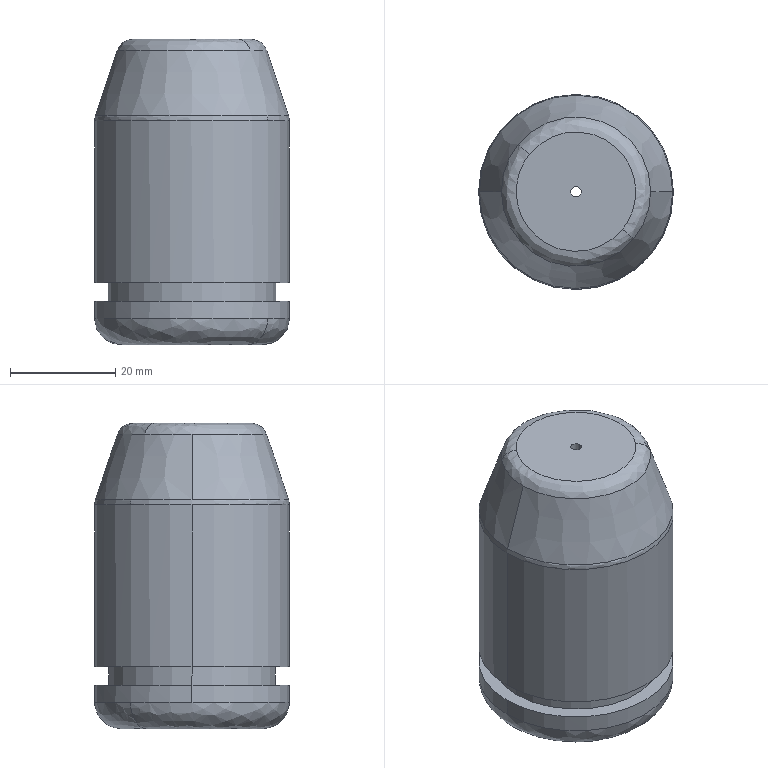Part | SolidWorks | features BaseBody 1 | 1 solid | 23 faces | box 37 x 37 x 58 mm | volume 55664 mm3 | cylinder 10 | spline 6 | plane 5 | cone 2 | commonest cylinder face diameters 37 x4 2 x2 5 x2 31.8 x2
STEP:
#1=CARTESIAN_POINT('',(495.143,-122.508,308.325));
#2=VERTEX_POINT('',#1);
#3=CARTESIAN_POINT('',(527.996,-134.18,308.325));
#4=VERTEX_POINT('',#3);
#5=CARTESIAN_POINT('',(509.496,-134.18,308.325));
#6=DIRECTION('',(-0.000000024,0.000000004,-1.));
#7=DIRECTION('',(-1.,0.,0.000000024));
#8=AXIS2_PLACEMENT_3D('',#5,#6,#7);
#9=CIRCLE('',#8,18.5);
#10=EDGE_CURVE('',#2,#4,#9,.T.);
#11=ORIENTED_EDGE('',*,*,#10,.F.);
#12=CARTESIAN_POINT('',(495.263,-122.605,309.274));
#13=VERTEX_POINT('',#12);
#14=CARTESIAN_POINT('',(497.471,-124.401,308.325));
#15=DIRECTION('',(0.6309,0.7758,-0.000000012));
#16=DIRECTION('',(-0.7758,0.6309,0.000000021));
#17=AXIS2_PLACEMENT_3D('',#14,#15,#16);
#18=CIRCLE('',#17,3.);
#19=EDGE_CURVE('',#2,#13,#18,.T.);
#20=ORIENTED_EDGE('',*,*,#19,.T.);
#21=CARTESIAN_POINT('',(527.842,-134.18,309.274));
#22=VERTEX_POINT('',#21);
#23=CARTESIAN_POINT('',(509.496,-134.18,309.274));
#24=DIRECTION('',(-0.000000024,0.000000004,-1.));
#25=DIRECTION('',(0.7758,-0.6309,-0.000000021));
#26=AXIS2_PLACEMENT_3D('',#23,#24,#25);
#27=CIRCLE('',#26,18.346);
#28=EDGE_CURVE('',#13,#22,#27,.T.);
#29=ORIENTED_EDGE('',*,*,#28,.T.);
#30=CARTESIAN_POINT('',(523.73,-145.756,309.274));
#31=VERTEX_POINT('',#30);
#32=CARTESIAN_POINT('',(509.496,-134.18,309.274));
#33=DIRECTION('',(-0.000000024,0.000000004,-1.));
#34=DIRECTION('',(0.7758,-0.6309,-0.000000021));
#35=AXIS2_PLACEMENT_3D('',#32,#33,#34);
#36=CIRCLE('',#35,18.346);
#37=EDGE_CURVE('',#22,#31,#36,.T.);
#38=ORIENTED_EDGE('',*,*,#37,.T.);
#39=CARTESIAN_POINT('',(523.849,-145.853,308.325));
#40=VERTEX_POINT('',#39);
#41=CARTESIAN_POINT('',(521.522,-143.96,308.325));
#42=DIRECTION('',(-0.6309,-0.7758,0.000000012));
#43=DIRECTION('',(0.7758,-0.6309,-0.000000021));
#44=AXIS2_PLACEMENT_3D('',#41,#42,#43);
#45=CIRCLE('',#44,3.);
#46=EDGE_CURVE('',#40,#31,#45,.T.);
#47=ORIENTED_EDGE('',*,*,#46,.F.);
#48=CARTESIAN_POINT('',(509.496,-134.18,308.325));
#49=DIRECTION('',(-0.000000024,0.000000004,-1.));
#50=DIRECTION('',(-1.,0.,0.000000024));
#51=AXIS2_PLACEMENT_3D('',#48,#49,#50);
#52=CIRCLE('',#51,18.5);
#53=EDGE_CURVE('',#4,#40,#52,.T.);
#54=ORIENTED_EDGE('',*,*,#53,.F.);
#55=EDGE_LOOP('',(#11,#20,#29,#38,#47,#54));
#56=FACE_OUTER_BOUND('',#55,.T.);
#57=CARTESIAN_POINT('',(495.143,-122.508,308.325));
#58=CARTESIAN_POINT('',(518.488,-93.802,308.325));
#59=CARTESIAN_POINT('',(547.194,-117.147,308.325));
#60=CARTESIAN_POINT('',(523.849,-145.853,308.325));
#61=CARTESIAN_POINT('',(495.143,-122.508,308.648));
#62=CARTESIAN_POINT('',(518.488,-93.802,308.648));
#63=CARTESIAN_POINT('',(547.194,-117.147,308.648));
#64=CARTESIAN_POINT('',(523.849,-145.853,308.648));
#65=CARTESIAN_POINT('',(495.183,-122.541,308.967));
#66=CARTESIAN_POINT('',(518.462,-93.915,308.967));
#67=CARTESIAN_POINT('',(547.088,-117.194,308.967));
#68=CARTESIAN_POINT('',(523.809,-145.82,308.967));
#69=CARTESIAN_POINT('',(495.263,-122.605,309.274));
#70=CARTESIAN_POINT('',(518.413,-94.138,309.274));
#71=CARTESIAN_POINT('',(546.88,-117.288,309.274));
#72=CARTESIAN_POINT('',(523.73,-145.756,309.274));
#73=(BOUNDED_SURFACE()B_SPLINE_SURFACE(3,3,((#57,#58,#59,#60),(#61,#62,#63,#64),(#65,#66,#67,#68),(#69,#70,#71,#72)),.UNSPECIFIED.,.F.,.F.,.T.)B_SPLINE_SURFACE_WITH_KNOTS((4,4),(4,4),(0.,1.),(0.,1.),.UNSPECIFIED.)GEOMETRIC_REPRESENTATION_ITEM()RATIONAL_B_SPLINE_SURFACE(((1.,0.3333,0.3333,1.),(0.9914,0.3305,0.3305,0.9914),(0.9914,0.3305,0.3305,0.9914),(1.,0.3333,0.3333,1.)))REPRESENTATION_ITEM('')SURFACE());
#74=ADVANCED_FACE('',(#56),#73,.T.);
#75=CARTESIAN_POINT('',(518.292,-141.334,323.812));
#76=VERTEX_POINT('',#75);
#77=CARTESIAN_POINT('',(500.7,-127.027,323.812));
#78=VERTEX_POINT('',#77);
#79=CARTESIAN_POINT('',(518.292,-141.334,323.812));
#80=CARTESIAN_POINT('',(503.986,-158.926,323.812));
#81=CARTESIAN_POINT('',(486.393,-144.62,323.812));
#82=CARTESIAN_POINT('',(500.7,-127.027,323.812));
#83=(BOUNDED_CURVE()B_SPLINE_CURVE(3,(#79,#80,#81,#82),.UNSPECIFIED.,.F.,.T.)B_SPLINE_CURVE_WITH_KNOTS((4,4),(0.,1.),.UNSPECIFIED.)CURVE()GEOMETRIC_REPRESENTATION_ITEM()RATIONAL_B_SPLINE_CURVE((1.,0.3333,0.3333,1.))REPRESENTATION_ITEM(''));
#84=EDGE_CURVE('',#76,#78,#83,.T.);
#85=ORIENTED_EDGE('',*,*,#84,.T.);
#86=CARTESIAN_POINT('',(498.492,-125.232,321.761));
#87=VERTEX_POINT('',#86);
#88=CARTESIAN_POINT('',(500.7,-127.027,320.812));
#89=DIRECTION('',(-0.6309,-0.7758,0.000000012));
#90=DIRECTION('',(-0.7758,0.6309,0.000000021));
#91=AXIS2_PLACEMENT_3D('',#88,#89,#90);
#92=CIRCLE('',#91,3.);
#93=EDGE_CURVE('',#78,#87,#92,.T.);
#94=ORIENTED_EDGE('',*,*,#93,.T.);
#95=CARTESIAN_POINT('',(495.312,-134.18,321.761));
#96=VERTEX_POINT('',#95);
#97=CARTESIAN_POINT('',(509.496,-134.18,321.761));
#98=DIRECTION('',(-0.000000024,0.000000004,-1.));
#99=DIRECTION('',(0.7758,-0.6309,-0.000000021));
#100=AXIS2_PLACEMENT_3D('',#97,#98,#99);
#101=CIRCLE('',#100,14.184);
#102=EDGE_CURVE('',#96,#87,#101,.T.);
#103=ORIENTED_EDGE('',*,*,#102,.F.);
#104=CARTESIAN_POINT('',(520.501,-143.129,321.761));
#105=VERTEX_POINT('',#104);
#106=CARTESIAN_POINT('',(509.496,-134.18,321.761));
#107=DIRECTION('',(-0.000000024,0.000000004,-1.));
#108=DIRECTION('',(0.7758,-0.6309,-0.000000021));
#109=AXIS2_PLACEMENT_3D('',#106,#107,#108);
#110=CIRCLE('',#109,14.184);
#111=EDGE_CURVE('',#105,#96,#110,.T.);
#112=ORIENTED_EDGE('',*,*,#111,.F.);
#113=CARTESIAN_POINT('',(518.292,-141.334,320.812));
#114=DIRECTION('',(0.6309,0.7758,-0.000000012));
#115=DIRECTION('',(0.7758,-0.6309,-0.000000021));
#116=AXIS2_PLACEMENT_3D('',#113,#114,#115);
#117=CIRCLE('',#116,3.);
#118=EDGE_CURVE('',#76,#105,#117,.T.);
#119=ORIENTED_EDGE('',*,*,#118,.F.);
#120=EDGE_LOOP('',(#85,#94,#103,#112,#119));
#121=FACE_OUTER_BOUND('',#120,.T.);
#122=CARTESIAN_POINT('',(500.7,-127.027,323.812));
#123=CARTESIAN_POINT('',(486.393,-144.62,323.812));
#124=CARTESIAN_POINT('',(503.986,-158.926,323.812));
#125=CARTESIAN_POINT('',(518.292,-141.334,323.812));
#126=CARTESIAN_POINT('',(499.662,-126.183,323.812));
#127=CARTESIAN_POINT('',(483.667,-145.851,323.812));
#128=CARTESIAN_POINT('',(503.336,-161.846,323.812));
#129=CARTESIAN_POINT('',(519.33,-142.178,323.812));
#130=CARTESIAN_POINT('',(498.82,-125.498,323.03));
#131=CARTESIAN_POINT('',(481.456,-146.851,323.03));
#132=CARTESIAN_POINT('',(502.808,-164.215,323.03));
#133=CARTESIAN_POINT('',(520.172,-142.863,323.03));
#134=CARTESIAN_POINT('',(498.492,-125.232,321.761));
#135=CARTESIAN_POINT('',(480.594,-147.24,321.761));
#136=CARTESIAN_POINT('',(502.603,-165.138,321.761));
#137=CARTESIAN_POINT('',(520.501,-143.129,321.761));
#138=(BOUNDED_SURFACE()B_SPLINE_SURFACE(3,3,((#122,#123,#124,#125),(#126,#127,#128,#129),(#130,#131,#132,#133),(#134,#135,#136,#137)),.UNSPECIFIED.,.F.,.F.,.F.)B_SPLINE_SURFACE_WITH_KNOTS((4,4),(4,4),(0.,1.),(0.,1.),.UNSPECIFIED.)GEOMETRIC_REPRESENTATION_ITEM()RATIONAL_B_SPLINE_SURFACE(((1.,0.3333,0.3333,1.),(0.8742,0.2914,0.2914,0.8742),(0.8742,0.2914,0.2914,0.8742),(1.,0.3333,0.3333,1.)))REPRESENTATION_ITEM('')SURFACE());
#139=ADVANCED_FACE('',(#121),#138,.T.);
#140=CARTESIAN_POINT('',(519.97,-142.698,265.812));
#141=VERTEX_POINT('',#140);
#142=CARTESIAN_POINT('',(499.022,-125.663,265.812));
#143=VERTEX_POINT('',#142);
#144=CARTESIAN_POINT('',(519.97,-142.698,265.812));
#145=CARTESIAN_POINT('',(537.005,-121.75,265.812));
#146=CARTESIAN_POINT('',(516.057,-104.715,265.812));
#147=CARTESIAN_POINT('',(499.022,-125.663,265.812));
#148=(BOUNDED_CURVE()B_SPLINE_CURVE(3,(#144,#145,#146,#147),.UNSPECIFIED.,.F.,.F.)B_SPLINE_CURVE_WITH_KNOTS((4,4),(0.,1.),.UNSPECIFIED.)CURVE()GEOMETRIC_REPRESENTATION_ITEM()RATIONAL_B_SPLINE_CURVE((1.,0.3333,0.3333,1.))REPRESENTATION_ITEM(''));
#149=EDGE_CURVE('',#141,#143,#148,.T.);
#150=ORIENTED_EDGE('',*,*,#149,.T.);
#151=CARTESIAN_POINT('',(495.143,-122.508,270.812));
#152=VERTEX_POINT('',#151);
#153=CARTESIAN_POINT('',(499.022,-125.663,270.812));
#154=DIRECTION('',(0.6309,0.7758,-0.000000012));
#155=DIRECTION('',(-0.7758,0.6309,0.000000021));
#156=AXIS2_PLACEMENT_3D('',#153,#154,#155);
#157=CIRCLE('',#156,5.);
#158=EDGE_CURVE('',#143,#152,#157,.T.);
#159=ORIENTED_EDGE('',*,*,#158,.T.);
#160=CARTESIAN_POINT('',(527.996,-134.18,270.812));
#161=VERTEX_POINT('',#160);
#162=CARTESIAN_POINT('',(509.496,-134.18,270.812));
#163=DIRECTION('',(0.000000024,-0.000000004,1.));
#164=DIRECTION('',(-1.,0.,0.000000024));
#165=AXIS2_PLACEMENT_3D('',#162,#163,#164);
#166=CIRCLE('',#165,18.5);
#167=EDGE_CURVE('',#161,#152,#166,.T.);
#168=ORIENTED_EDGE('',*,*,#167,.F.);
#169=CARTESIAN_POINT('',(523.849,-145.853,270.812));
#170=VERTEX_POINT('',#169);
#171=CARTESIAN_POINT('',(509.496,-134.18,270.812));
#172=DIRECTION('',(0.000000024,-0.000000004,1.));
#173=DIRECTION('',(-1.,0.,0.000000024));
#174=AXIS2_PLACEMENT_3D('',#171,#172,#173);
#175=CIRCLE('',#174,18.5);
#176=EDGE_CURVE('',#170,#161,#175,.T.);
#177=ORIENTED_EDGE('',*,*,#176,.F.);
#178=CARTESIAN_POINT('',(519.97,-142.698,270.812));
#179=DIRECTION('',(-0.6309,-0.7758,0.000000012));
#180=DIRECTION('',(0.7758,-0.6309,-0.000000021));
#181=AXIS2_PLACEMENT_3D('',#178,#179,#180);
#182=CIRCLE('',#181,5.);
#183=EDGE_CURVE('',#141,#170,#182,.T.);
#184=ORIENTED_EDGE('',*,*,#183,.F.);
#185=EDGE_LOOP('',(#150,#159,#168,#177,#184));
#186=FACE_OUTER_BOUND('',#185,.T.);
#187=CARTESIAN_POINT('',(499.022,-125.663,265.812));
#188=CARTESIAN_POINT('',(516.057,-104.715,265.812));
#189=CARTESIAN_POINT('',(537.005,-121.75,265.812));
#190=CARTESIAN_POINT('',(519.97,-142.698,265.812));
#191=CARTESIAN_POINT('',(496.75,-123.815,265.812));
#192=CARTESIAN_POINT('',(517.481,-98.323,265.812));
#193=CARTESIAN_POINT('',(542.973,-119.054,265.812));
#194=CARTESIAN_POINT('',(522.242,-144.546,265.812));
#195=CARTESIAN_POINT('',(495.143,-122.508,267.883));
#196=CARTESIAN_POINT('',(518.488,-93.802,267.883));
#197=CARTESIAN_POINT('',(547.194,-117.147,267.883));
#198=CARTESIAN_POINT('',(523.849,-145.853,267.883));
#199=CARTESIAN_POINT('',(495.143,-122.508,270.812));
#200=CARTESIAN_POINT('',(518.488,-93.802,270.812));
#201=CARTESIAN_POINT('',(547.194,-117.147,270.812));
#202=CARTESIAN_POINT('',(523.849,-145.853,270.812));
#203=(BOUNDED_SURFACE()B_SPLINE_SURFACE(3,3,((#187,#188,#189,#190),(#191,#192,#193,#194),(#195,#196,#197,#198),(#199,#200,#201,#202)),.UNSPECIFIED.,.F.,.F.,.F.)B_SPLINE_SURFACE_WITH_KNOTS((4,4),(4,4),(0.,1.),(0.,1.),.UNSPECIFIED.)GEOMETRIC_REPRESENTATION_ITEM()RATIONAL_B_SPLINE_SURFACE(((1.,0.3333,0.3333,1.),(0.8047,0.2682,0.2682,0.8047),(0.8047,0.2682,0.2682,0.8047),(1.,0.3333,0.3333,1.)))REPRESENTATION_ITEM('')SURFACE());
#204=ADVANCED_FACE('',(#186),#203,.T.);
#205=CARTESIAN_POINT('',(490.996,-134.18,308.325));
#206=VERTEX_POINT('',#205);
#207=CARTESIAN_POINT('',(509.496,-134.18,308.325));
#208=DIRECTION('',(-0.000000024,0.000000004,-1.));
#209=DIRECTION('',(-1.,0.,0.000000024));
#210=AXIS2_PLACEMENT_3D('',#207,#208,#209);
#211=CIRCLE('',#210,18.5);
#212=EDGE_CURVE('',#206,#2,#211,.T.);
#213=ORIENTED_EDGE('',*,*,#212,.T.);
#214=ORIENTED_EDGE('',*,*,#10,.T.);
#215=CARTESIAN_POINT('',(527.996,-134.18,277.565));
#216=VERTEX_POINT('',#215);
#217=CARTESIAN_POINT('',(527.996,-134.18,323.812));
#218=DIRECTION('',(-0.000000024,0.000000004,-1.));
#219=VECTOR('',#218,1000.);
#220=LINE('',#217,#219);
#221=EDGE_CURVE('',#4,#216,#220,.T.);
#222=ORIENTED_EDGE('',*,*,#221,.T.);
#223=CARTESIAN_POINT('',(490.996,-134.18,277.565));
#224=VERTEX_POINT('',#223);
#225=CARTESIAN_POINT('',(509.496,-134.18,277.565));
#226=DIRECTION('',(0.000000024,-0.000000004,1.));
#227=DIRECTION('',(-1.,0.,0.000000024));
#228=AXIS2_PLACEMENT_3D('',#225,#226,#227);
#229=CIRCLE('',#228,18.5);
#230=EDGE_CURVE('',#216,#224,#229,.T.);
#231=ORIENTED_EDGE('',*,*,#230,.T.);
#232=CARTESIAN_POINT('',(490.996,-134.18,323.812));
#233=DIRECTION('',(-0.000000024,0.000000004,-1.));
#234=VECTOR('',#233,1000.);
#235=LINE('',#232,#234);
#236=EDGE_CURVE('',#206,#224,#235,.T.);
#237=ORIENTED_EDGE('',*,*,#236,.F.);
#238=EDGE_LOOP('',(#213,#214,#222,#231,#237));
#239=FACE_OUTER_BOUND('',#238,.T.);
#240=CARTESIAN_POINT('',(509.496,-134.18,323.812));
#241=DIRECTION('',(-0.000000024,0.000000004,-1.));
#242=DIRECTION('',(-1.,0.,0.000000024));
#243=AXIS2_PLACEMENT_3D('',#240,#241,#242);
#244=CYLINDRICAL_SURFACE('',#243,18.5);
#245=ADVANCED_FACE('',(#239),#244,.T.);
#246=CARTESIAN_POINT('',(493.596,-134.18,277.565));
#247=VERTEX_POINT('',#246);
#248=CARTESIAN_POINT('',(525.396,-134.18,277.565));
#249=VERTEX_POINT('',#248);
#250=CARTESIAN_POINT('',(509.496,-134.18,277.565));
#251=DIRECTION('',(-0.000000024,0.000000004,-1.));
#252=DIRECTION('',(-1.,0.,0.000000024));
#253=AXIS2_PLACEMENT_3D('',#250,#251,#252);
#254=CIRCLE('',#253,15.9);
#255=EDGE_CURVE('',#247,#249,#254,.T.);
#256=ORIENTED_EDGE('',*,*,#255,.T.);
#257=CARTESIAN_POINT('',(525.396,-134.18,274.065));
#258=VERTEX_POINT('',#257);
#259=CARTESIAN_POINT('',(525.396,-134.18,275.815));
#260=DIRECTION('',(-0.000000024,0.000000004,-1.));
#261=VECTOR('',#260,1000.);
#262=LINE('',#259,#261);
#263=EDGE_CURVE('',#249,#258,#262,.T.);
#264=ORIENTED_EDGE('',*,*,#263,.T.);
#265=CARTESIAN_POINT('',(493.596,-134.18,274.065));
#266=VERTEX_POINT('',#265);
#267=CARTESIAN_POINT('',(509.496,-134.18,274.065));
#268=DIRECTION('',(0.000000024,-0.000000004,1.));
#269=DIRECTION('',(-1.,0.,0.000000024));
#270=AXIS2_PLACEMENT_3D('',#267,#268,#269);
#271=CIRCLE('',#270,15.9);
#272=EDGE_CURVE('',#258,#266,#271,.T.);
#273=ORIENTED_EDGE('',*,*,#272,.T.);
#274=CARTESIAN_POINT('',(493.596,-134.18,275.815));
#275=DIRECTION('',(-0.000000024,0.000000004,-1.));
#276=VECTOR('',#275,1000.);
#277=LINE('',#274,#276);
#278=EDGE_CURVE('',#247,#266,#277,.T.);
#279=ORIENTED_EDGE('',*,*,#278,.F.);
#280=EDGE_LOOP('',(#256,#264,#273,#279));
#281=FACE_OUTER_BOUND('',#280,.T.);
#282=CARTESIAN_POINT('',(509.496,-134.18,275.815));
#283=DIRECTION('',(-0.000000024,0.000000004,-1.));
#284=DIRECTION('',(-1.,0.,0.000000024));
#285=AXIS2_PLACEMENT_3D('',#282,#283,#284);
#286=CYLINDRICAL_SURFACE('',#285,15.9);
#287=ADVANCED_FACE('',(#281),#286,.T.);
#288=ORIENTED_EDGE('',*,*,#102,.T.);
#289=CARTESIAN_POINT('',(523.68,-134.18,321.761));
#290=VERTEX_POINT('',#289);
#291=CARTESIAN_POINT('',(509.496,-134.18,321.761));
#292=DIRECTION('',(-0.000000024,0.000000004,-1.));
#293=DIRECTION('',(0.7758,-0.6309,-0.000000021));
#294=AXIS2_PLACEMENT_3D('',#291,#292,#293);
#295=CIRCLE('',#294,14.184);
#296=EDGE_CURVE('',#87,#290,#295,.T.);
#297=ORIENTED_EDGE('',*,*,#296,.T.);
#298=CARTESIAN_POINT('',(527.842,-134.18,309.274));
#299=DIRECTION('',(0.3162,0.000000004,-0.9487));
#300=VECTOR('',#299,1000.);
#301=LINE('',#298,#300);
#302=EDGE_CURVE('',#290,#22,#301,.T.);
#303=ORIENTED_EDGE('',*,*,#302,.T.);
#304=ORIENTED_EDGE('',*,*,#28,.F.);
#305=CARTESIAN_POINT('',(491.15,-134.18,309.274));
#306=VERTEX_POINT('',#305);
#307=CARTESIAN_POINT('',(509.496,-134.18,309.274));
#308=DIRECTION('',(-0.000000024,0.000000004,-1.));
#309=DIRECTION('',(0.7758,-0.6309,-0.000000021));
#310=AXIS2_PLACEMENT_3D('',#307,#308,#309);
#311=CIRCLE('',#310,18.346);
#312=EDGE_CURVE('',#306,#13,#311,.T.);
#313=ORIENTED_EDGE('',*,*,#312,.F.);
#314=CARTESIAN_POINT('',(491.15,-134.18,309.274));
#315=DIRECTION('',(-0.3162,0.000000004,-0.9487));
#316=VECTOR('',#315,1000.);
#317=LINE('',#314,#316);
#318=EDGE_CURVE('',#96,#306,#317,.T.);
#319=ORIENTED_EDGE('',*,*,#318,.F.);
#320=EDGE_LOOP('',(#288,#297,#303,#304,#313,#319));
#321=FACE_OUTER_BOUND('',#320,.T.);
#322=CARTESIAN_POINT('',(509.496,-134.18,309.274));
#323=DIRECTION('',(-0.000000024,0.000000004,-1.));
#324=DIRECTION('',(-1.,0.,0.000000024));
#325=AXIS2_PLACEMENT_3D('',#322,#323,#324);
#326=CONICAL_SURFACE('',#325,18.346,0.3218);
#327=ADVANCED_FACE('',(#321),#326,.T.);
#328=CARTESIAN_POINT('',(490.996,-134.18,274.065));
#329=VERTEX_POINT('',#328);
#330=CARTESIAN_POINT('',(527.996,-134.18,274.065));
#331=VERTEX_POINT('',#330);
#332=CARTESIAN_POINT('',(509.496,-134.18,274.065));
#333=DIRECTION('',(-0.000000024,0.000000004,-1.));
#334=DIRECTION('',(-1.,0.,0.000000024));
#335=AXIS2_PLACEMENT_3D('',#332,#333,#334);
#336=CIRCLE('',#335,18.5);
#337=EDGE_CURVE('',#329,#331,#336,.T.);
#338=ORIENTED_EDGE('',*,*,#337,.T.);
#339=CARTESIAN_POINT('',(527.996,-134.18,323.812));
#340=DIRECTION('',(-0.000000024,0.000000004,-1.));
#341=VECTOR('',#340,1000.);
#342=LINE('',#339,#341);
#343=EDGE_CURVE('',#331,#161,#342,.T.);
#344=ORIENTED_EDGE('',*,*,#343,.T.);
#345=ORIENTED_EDGE('',*,*,#167,.T.);
#346=CARTESIAN_POINT('',(490.996,-134.18,270.812));
#347=VERTEX_POINT('',#346);
#348=CARTESIAN_POINT('',(509.496,-134.18,270.812));
#349=DIRECTION('',(0.000000024,-0.000000004,1.));
#350=DIRECTION('',(-1.,0.,0.000000024));
#351=AXIS2_PLACEMENT_3D('',#348,#349,#350);
#352=CIRCLE('',#351,18.5);
#353=EDGE_CURVE('',#152,#347,#352,.T.);
#354=ORIENTED_EDGE('',*,*,#353,.T.);
#355=CARTESIAN_POINT('',(490.996,-134.18,323.812));
#356=DIRECTION('',(-0.000000024,0.000000004,-1.));
#357=VECTOR('',#356,1000.);
#358=LINE('',#355,#357);
#359=EDGE_CURVE('',#329,#347,#358,.T.);
#360=ORIENTED_EDGE('',*,*,#359,.F.);
#361=EDGE_LOOP('',(#338,#344,#345,#354,#360));
#362=FACE_OUTER_BOUND('',#361,.T.);
#363=CARTESIAN_POINT('',(509.496,-134.18,323.812));
#364=DIRECTION('',(-0.000000024,0.000000004,-1.));
#365=DIRECTION('',(-1.,0.,0.000000024));
#366=AXIS2_PLACEMENT_3D('',#363,#364,#365);
#367=CYLINDRICAL_SURFACE('',#366,18.5);
#368=ADVANCED_FACE('',(#362),#367,.T.);
#369=CARTESIAN_POINT('',(508.496,-134.18,320.812));
#370=VERTEX_POINT('',#369);
#371=CARTESIAN_POINT('',(510.496,-134.18,320.812));
#372=VERTEX_POINT('',#371);
#373=CARTESIAN_POINT('',(509.496,-134.18,320.812));
#374=DIRECTION('',(0.000000024,-0.000000004,1.));
#375=DIRECTION('',(1.,0.,-0.000000024));
#376=AXIS2_PLACEMENT_3D('',#373,#374,#375);
#377=CIRCLE('',#376,1.);
#378=EDGE_CURVE('',#370,#372,#377,.T.);
#379=ORIENTED_EDGE('',*,*,#378,.F.);
#380=CARTESIAN_POINT('',(508.496,-134.18,323.812));
#381=VERTEX_POINT('',#380);
#382=CARTESIAN_POINT('',(508.496,-134.18,323.812));
#383=DIRECTION('',(0.000000024,-0.000000004,1.));
#384=VECTOR('',#383,1000.);
#385=LINE('',#382,#384);
#386=EDGE_CURVE('',#370,#381,#385,.T.);
#387=ORIENTED_EDGE('',*,*,#386,.T.);
#388=CARTESIAN_POINT('',(510.496,-134.18,323.812));
#389=VERTEX_POINT('',#388);
#390=CARTESIAN_POINT('',(509.496,-134.18,323.812));
#391=DIRECTION('',(0.000000024,-0.000000004,1.));
#392=DIRECTION('',(1.,0.,-0.000000024));
#393=AXIS2_PLACEMENT_3D('',#390,#391,#392);
#394=CIRCLE('',#393,1.);
#395=EDGE_CURVE('',#381,#389,#394,.T.);
#396=ORIENTED_EDGE('',*,*,#395,.T.);
#397=CARTESIAN_POINT('',(510.496,-134.18,323.812));
#398=DIRECTION('',(0.000000024,-0.000000004,1.));
#399=VECTOR('',#398,1000.);
#400=LINE('',#397,#399);
#401=EDGE_CURVE('',#372,#389,#400,.T.);
#402=ORIENTED_EDGE('',*,*,#401,.F.);
#403=EDGE_LOOP('',(#379,#387,#396,#402));
#404=FACE_OUTER_BOUND('',#403,.T.);
#405=CARTESIAN_POINT('',(509.496,-134.18,323.812));
#406=DIRECTION('',(0.000000024,-0.000000004,1.));
#407=DIRECTION('',(1.,0.,-0.000000024));
#408=AXIS2_PLACEMENT_3D('',#405,#406,#407);
#409=CYLINDRICAL_SURFACE('',#408,1.);
#410=ADVANCED_FACE('',(#404),#409,.F.);
#411=CARTESIAN_POINT('',(506.996,-134.18,320.812));
#412=VERTEX_POINT('',#411);
#413=CARTESIAN_POINT('',(511.996,-134.18,320.812));
#414=VERTEX_POINT('',#413);
#415=CARTESIAN_POINT('',(509.496,-134.18,320.812));
#416=DIRECTION('',(0.000000024,-0.000000004,1.));
#417=DIRECTION('',(-1.,0.,0.000000024));
#418=AXIS2_PLACEMENT_3D('',#415,#416,#417);
#419=CIRCLE('',#418,2.5);
#420=EDGE_CURVE('',#412,#414,#419,.T.);
#421=ORIENTED_EDGE('',*,*,#420,.T.);
#422=CARTESIAN_POINT('',(511.996,-134.18,265.812));
#423=VERTEX_POINT('',#422);
#424=CARTESIAN_POINT('',(511.996,-134.18,265.812));
#425=DIRECTION('',(-0.000000024,0.000000004,-1.));
#426=VECTOR('',#425,1000.);
#427=LINE('',#424,#426);
#428=EDGE_CURVE('',#414,#423,#427,.T.);
#429=ORIENTED_EDGE('',*,*,#428,.T.);
#430=CARTESIAN_POINT('',(506.996,-134.18,265.812));
#431=VERTEX_POINT('',#430);
#432=CARTESIAN_POINT('',(509.496,-134.18,265.812));
#433=DIRECTION('',(0.000000024,-0.000000004,1.));
#434=DIRECTION('',(-1.,0.,0.000000024));
#435=AXIS2_PLACEMENT_3D('',#432,#433,#434);
#436=CIRCLE('',#435,2.5);
#437=EDGE_CURVE('',#431,#423,#436,.T.);
#438=ORIENTED_EDGE('',*,*,#437,.F.);
#439=CARTESIAN_POINT('',(506.996,-134.18,265.812));
#440=DIRECTION('',(-0.000000024,0.000000004,-1.));
#441=VECTOR('',#440,1000.);
#442=LINE('',#439,#441);
#443=EDGE_CURVE('',#412,#431,#442,.T.);
#444=ORIENTED_EDGE('',*,*,#443,.F.);
#445=EDGE_LOOP('',(#421,#429,#438,#444));
#446=FACE_OUTER_BOUND('',#445,.T.);
#447=CARTESIAN_POINT('',(509.496,-134.18,265.812));
#448=DIRECTION('',(-0.000000024,0.000000004,-1.));
#449=DIRECTION('',(-1.,0.,0.000000024));
#450=AXIS2_PLACEMENT_3D('',#447,#448,#449);
#451=CYLINDRICAL_SURFACE('',#450,2.5);
#452=ADVANCED_FACE('',(#446),#451,.F.);
#453=ORIENTED_EDGE('',*,*,#221,.F.);
#454=ORIENTED_EDGE('',*,*,#53,.T.);
#455=CARTESIAN_POINT('',(509.496,-134.18,308.325));
#456=DIRECTION('',(-0.000000024,0.000000004,-1.));
#457=DIRECTION('',(-1.,0.,0.000000024));
#458=AXIS2_PLACEMENT_3D('',#455,#456,#457);
#459=CIRCLE('',#458,18.5);
#460=EDGE_CURVE('',#40,#206,#459,.T.);
#461=ORIENTED_EDGE('',*,*,#460,.T.);
#462=ORIENTED_EDGE('',*,*,#236,.T.);
#463=CARTESIAN_POINT('',(509.496,-134.18,277.565));
#464=DIRECTION('',(0.000000024,-0.000000004,1.));
#465=DIRECTION('',(-1.,0.,0.000000024));
#466=AXIS2_PLACEMENT_3D('',#463,#464,#465);
#467=CIRCLE('',#466,18.5);
#468=EDGE_CURVE('',#224,#216,#467,.T.);
#469=ORIENTED_EDGE('',*,*,#468,.T.);
#470=EDGE_LOOP('',(#453,#454,#461,#462,#469));
#471=FACE_OUTER_BOUND('',#470,.T.);
#472=CARTESIAN_POINT('',(509.496,-134.18,323.812));
#473=DIRECTION('',(-0.000000024,0.000000004,-1.));
#474=DIRECTION('',(-1.,0.,0.000000024));
#475=AXIS2_PLACEMENT_3D('',#472,#473,#474);
#476=CYLINDRICAL_SURFACE('',#475,18.5);
#477=ADVANCED_FACE('',(#471),#476,.T.);
#478=ORIENTED_EDGE('',*,*,#468,.F.);
#479=ORIENTED_EDGE('',*,*,#230,.F.);
#480=EDGE_LOOP('',(#478,#479));
#481=FACE_OUTER_BOUND('',#480,.T.);
#482=ORIENTED_EDGE('',*,*,#255,.F.);
#483=CARTESIAN_POINT('',(509.496,-134.18,277.565));
#484=DIRECTION('',(-0.000000024,0.000000004,-1.));
#485=DIRECTION('',(-1.,0.,0.000000024));
#486=AXIS2_PLACEMENT_3D('',#483,#484,#485);
#487=CIRCLE('',#486,15.9);
#488=EDGE_CURVE('',#249,#247,#487,.T.);
#489=ORIENTED_EDGE('',*,*,#488,.F.);
#490=EDGE_LOOP('',(#482,#489));
#491=FACE_BOUND('',#490,.T.);
#492=CARTESIAN_POINT('',(496.152,-123.329,277.565));
#493=DIRECTION('',(0.000000024,-0.000000004,1.));
#494=DIRECTION('',(1.,0.,-0.000000024));
#495=AXIS2_PLACEMENT_3D('',#492,#493,#494);
#496=PLANE('',#495);
#497=ADVANCED_FACE('',(#481,#491),#496,.F.);
#498=ORIENTED_EDGE('',*,*,#19,.F.);
#499=ORIENTED_EDGE('',*,*,#212,.F.);
#500=ORIENTED_EDGE('',*,*,#460,.F.);
#501=ORIENTED_EDGE('',*,*,#46,.T.);
#502=CARTESIAN_POINT('',(509.496,-134.18,309.274));
#503=DIRECTION('',(-0.000000024,0.000000004,-1.));
#504=DIRECTION('',(0.7758,-0.6309,-0.000000021));
#505=AXIS2_PLACEMENT_3D('',#502,#503,#504);
#506=CIRCLE('',#505,18.346);
#507=EDGE_CURVE('',#31,#306,#506,.T.);
#508=ORIENTED_EDGE('',*,*,#507,.T.);
#509=ORIENTED_EDGE('',*,*,#312,.T.);
#510=EDGE_LOOP('',(#498,#499,#500,#501,#508,#509));
#511=FACE_OUTER_BOUND('',#510,.T.);
#512=CARTESIAN_POINT('',(523.849,-145.853,308.325));
#513=CARTESIAN_POINT('',(500.505,-174.559,308.325));
#514=CARTESIAN_POINT('',(471.799,-151.214,308.325));
#515=CARTESIAN_POINT('',(495.143,-122.508,308.325));
#516=CARTESIAN_POINT('',(523.849,-145.853,308.648));
#517=CARTESIAN_POINT('',(500.505,-174.559,308.648));
#518=CARTESIAN_POINT('',(471.799,-151.214,308.648));
#519=CARTESIAN_POINT('',(495.143,-122.508,308.648));
#520=CARTESIAN_POINT('',(523.809,-145.82,308.967));
#521=CARTESIAN_POINT('',(500.53,-174.446,308.967));
#522=CARTESIAN_POINT('',(471.904,-151.167,308.967));
#523=CARTESIAN_POINT('',(495.183,-122.541,308.967));
#524=CARTESIAN_POINT('',(523.73,-145.756,309.274));
#525=CARTESIAN_POINT('',(500.58,-174.223,309.274));
#526=CARTESIAN_POINT('',(472.112,-151.073,309.274));
#527=CARTESIAN_POINT('',(495.263,-122.605,309.274));
#528=(BOUNDED_SURFACE()B_SPLINE_SURFACE(3,3,((#512,#513,#514,#515),(#516,#517,#518,#519),(#520,#521,#522,#523),(#524,#525,#526,#527)),.UNSPECIFIED.,.F.,.F.,.T.)B_SPLINE_SURFACE_WITH_KNOTS((4,4),(4,4),(0.,1.),(0.,1.),.UNSPECIFIED.)GEOMETRIC_REPRESENTATION_ITEM()RATIONAL_B_SPLINE_SURFACE(((1.,0.3333,0.3333,1.),(0.9914,0.3305,0.3305,0.9914),(0.9914,0.3305,0.3305,0.9914),(1.,0.3333,0.3333,1.)))REPRESENTATION_ITEM('')SURFACE());
#529=ADVANCED_FACE('',(#511),#528,.T.);
#530=ORIENTED_EDGE('',*,*,#263,.F.);
#531=ORIENTED_EDGE('',*,*,#488,.T.);
#532=ORIENTED_EDGE('',*,*,#278,.T.);
#533=CARTESIAN_POINT('',(509.496,-134.18,274.065));
#534=DIRECTION('',(0.000000024,-0.000000004,1.));
#535=DIRECTION('',(-1.,0.,0.000000024));
#536=AXIS2_PLACEMENT_3D('',#533,#534,#535);
#537=CIRCLE('',#536,15.9);
#538=EDGE_CURVE('',#266,#258,#537,.T.);
#539=ORIENTED_EDGE('',*,*,#538,.T.);
#540=EDGE_LOOP('',(#530,#531,#532,#539));
#541=FACE_OUTER_BOUND('',#540,.T.);
#542=CARTESIAN_POINT('',(509.496,-134.18,275.815));
#543=DIRECTION('',(-0.000000024,0.000000004,-1.));
#544=DIRECTION('',(-1.,0.,0.000000024));
#545=AXIS2_PLACEMENT_3D('',#542,#543,#544);
#546=CYLINDRICAL_SURFACE('',#545,15.9);
#547=ADVANCED_FACE('',(#541),#546,.T.);
#548=ORIENTED_EDGE('',*,*,#302,.F.);
#549=CARTESIAN_POINT('',(509.496,-134.18,321.761));
#550=DIRECTION('',(-0.000000024,0.000000004,-1.));
#551=DIRECTION('',(0.7758,-0.6309,-0.000000021));
#552=AXIS2_PLACEMENT_3D('',#549,#550,#551);
#553=CIRCLE('',#552,14.184);
#554=EDGE_CURVE('',#290,#105,#553,.T.);
#555=ORIENTED_EDGE('',*,*,#554,.T.);
#556=ORIENTED_EDGE('',*,*,#111,.T.);
#557=ORIENTED_EDGE('',*,*,#318,.T.);
#558=ORIENTED_EDGE('',*,*,#507,.F.);
#559=ORIENTED_EDGE('',*,*,#37,.F.);
#560=EDGE_LOOP('',(#548,#555,#556,#557,#558,#559));
#561=FACE_OUTER_BOUND('',#560,.T.);
#562=CARTESIAN_POINT('',(509.496,-134.18,309.274));
#563=DIRECTION('',(-0.000000024,0.000000004,-1.));
#564=DIRECTION('',(-1.,0.,0.000000024));
#565=AXIS2_PLACEMENT_3D('',#562,#563,#564);
#566=CONICAL_SURFACE('',#565,18.346,0.3218);
#567=ADVANCED_FACE('',(#561),#566,.T.);
#568=ORIENTED_EDGE('',*,*,#538,.F.);
#569=ORIENTED_EDGE('',*,*,#272,.F.);
#570=EDGE_LOOP('',(#568,#569));
#571=FACE_BOUND('',#570,.T.);
#572=ORIENTED_EDGE('',*,*,#337,.F.);
#573=CARTESIAN_POINT('',(509.496,-134.18,274.065));
#574=DIRECTION('',(-0.000000024,0.000000004,-1.));
#575=DIRECTION('',(-1.,0.,0.000000024));
#576=AXIS2_PLACEMENT_3D('',#573,#574,#575);
#577=CIRCLE('',#576,18.5);
#578=EDGE_CURVE('',#331,#329,#577,.T.);
#579=ORIENTED_EDGE('',*,*,#578,.F.);
#580=EDGE_LOOP('',(#572,#579));
#581=FACE_OUTER_BOUND('',#580,.T.);
#582=CARTESIAN_POINT('',(496.152,-123.329,274.065));
#583=DIRECTION('',(-0.000000024,0.000000004,-1.));
#584=DIRECTION('',(-1.,0.,0.000000024));
#585=AXIS2_PLACEMENT_3D('',#582,#583,#584);
#586=PLANE('',#585);
#587=ADVANCED_FACE('',(#571,#581),#586,.F.);
#588=ORIENTED_EDGE('',*,*,#93,.F.);
#589=CARTESIAN_POINT('',(500.7,-127.027,323.812));
#590=CARTESIAN_POINT('',(515.007,-109.435,323.812));
#591=CARTESIAN_POINT('',(532.599,-123.741,323.812));
#592=CARTESIAN_POINT('',(518.292,-141.334,323.812));
#593=(BOUNDED_CURVE()B_SPLINE_CURVE(3,(#589,#590,#591,#592),.UNSPECIFIED.,.F.,.T.)B_SPLINE_CURVE_WITH_KNOTS((4,4),(0.,1.),.UNSPECIFIED.)CURVE()GEOMETRIC_REPRESENTATION_ITEM()RATIONAL_B_SPLINE_CURVE((1.,0.3333,0.3333,1.))REPRESENTATION_ITEM(''));
#594=EDGE_CURVE('',#78,#76,#593,.T.);
#595=ORIENTED_EDGE('',*,*,#594,.T.);
#596=ORIENTED_EDGE('',*,*,#118,.T.);
#597=ORIENTED_EDGE('',*,*,#554,.F.);
#598=ORIENTED_EDGE('',*,*,#296,.F.);
#599=EDGE_LOOP('',(#588,#595,#596,#597,#598));
#600=FACE_OUTER_BOUND('',#599,.T.);
#601=CARTESIAN_POINT('',(518.292,-141.334,323.812));
#602=CARTESIAN_POINT('',(532.599,-123.741,323.812));
#603=CARTESIAN_POINT('',(515.007,-109.435,323.812));
#604=CARTESIAN_POINT('',(500.7,-127.027,323.812));
#605=CARTESIAN_POINT('',(519.33,-142.178,323.812));
#606=CARTESIAN_POINT('',(535.325,-122.51,323.812));
#607=CARTESIAN_POINT('',(515.657,-106.515,323.812));
#608=CARTESIAN_POINT('',(499.662,-126.183,323.812));
#609=CARTESIAN_POINT('',(520.172,-142.863,323.03));
#610=CARTESIAN_POINT('',(537.536,-121.51,323.03));
#611=CARTESIAN_POINT('',(516.184,-104.146,323.03));
#612=CARTESIAN_POINT('',(498.82,-125.498,323.03));
#613=CARTESIAN_POINT('',(520.501,-143.129,321.761));
#614=CARTESIAN_POINT('',(538.398,-121.121,321.761));
#615=CARTESIAN_POINT('',(516.39,-103.223,321.761));
#616=CARTESIAN_POINT('',(498.492,-125.232,321.761));
#617=(BOUNDED_SURFACE()B_SPLINE_SURFACE(3,3,((#601,#602,#603,#604),(#605,#606,#607,#608),(#609,#610,#611,#612),(#613,#614,#615,#616)),.UNSPECIFIED.,.F.,.F.,.F.)B_SPLINE_SURFACE_WITH_KNOTS((4,4),(4,4),(0.,1.),(0.,1.),.UNSPECIFIED.)GEOMETRIC_REPRESENTATION_ITEM()RATIONAL_B_SPLINE_SURFACE(((1.,0.3333,0.3333,1.),(0.8742,0.2914,0.2914,0.8742),(0.8742,0.2914,0.2914,0.8742),(1.,0.3333,0.3333,1.)))REPRESENTATION_ITEM('')SURFACE());
#618=ADVANCED_FACE('',(#600),#617,.T.);
#619=ORIENTED_EDGE('',*,*,#343,.F.);
#620=ORIENTED_EDGE('',*,*,#578,.T.);
#621=ORIENTED_EDGE('',*,*,#359,.T.);
#622=CARTESIAN_POINT('',(509.496,-134.18,270.812));
#623=DIRECTION('',(0.000000024,-0.000000004,1.));
#624=DIRECTION('',(-1.,0.,0.000000024));
#625=AXIS2_PLACEMENT_3D('',#622,#623,#624);
#626=CIRCLE('',#625,18.5);
#627=EDGE_CURVE('',#347,#170,#626,.T.);
#628=ORIENTED_EDGE('',*,*,#627,.T.);
#629=ORIENTED_EDGE('',*,*,#176,.T.);
#630=EDGE_LOOP('',(#619,#620,#621,#628,#629));
#631=FACE_OUTER_BOUND('',#630,.T.);
#632=CARTESIAN_POINT('',(509.496,-134.18,323.812));
#633=DIRECTION('',(-0.000000024,0.000000004,-1.));
#634=DIRECTION('',(-1.,0.,0.000000024));
#635=AXIS2_PLACEMENT_3D('',#632,#633,#634);
#636=CYLINDRICAL_SURFACE('',#635,18.5);
#637=ADVANCED_FACE('',(#631),#636,.T.);
#638=ORIENTED_EDGE('',*,*,#84,.F.);
#639=ORIENTED_EDGE('',*,*,#594,.F.);
#640=EDGE_LOOP('',(#638,#639));
#641=FACE_OUTER_BOUND('',#640,.T.);
#642=CARTESIAN_POINT('',(509.496,-134.18,323.812));
#643=DIRECTION('',(0.000000024,-0.000000004,1.));
#644=DIRECTION('',(1.,0.,-0.000000024));
#645=AXIS2_PLACEMENT_3D('',#642,#643,#644);
#646=CIRCLE('',#645,1.);
#647=EDGE_CURVE('',#389,#381,#646,.T.);
#648=ORIENTED_EDGE('',*,*,#647,.F.);
#649=ORIENTED_EDGE('',*,*,#395,.F.);
#650=EDGE_LOOP('',(#648,#649));
#651=FACE_BOUND('',#650,.T.);
#652=CARTESIAN_POINT('',(509.496,-134.18,323.812));
#653=DIRECTION('',(-0.000000024,0.000000004,-1.));
#654=DIRECTION('',(-1.,0.,0.000000024));
#655=AXIS2_PLACEMENT_3D('',#652,#653,#654);
#656=PLANE('',#655);
#657=ADVANCED_FACE('',(#641,#651),#656,.F.);
#658=ORIENTED_EDGE('',*,*,#158,.F.);
#659=CARTESIAN_POINT('',(499.022,-125.663,265.812));
#660=CARTESIAN_POINT('',(481.987,-146.611,265.812));
#661=CARTESIAN_POINT('',(502.935,-163.646,265.812));
#662=CARTESIAN_POINT('',(519.97,-142.698,265.812));
#663=(BOUNDED_CURVE()B_SPLINE_CURVE(3,(#659,#660,#661,#662),.UNSPECIFIED.,.F.,.F.)B_SPLINE_CURVE_WITH_KNOTS((4,4),(0.,1.),.UNSPECIFIED.)CURVE()GEOMETRIC_REPRESENTATION_ITEM()RATIONAL_B_SPLINE_CURVE((1.,0.3333,0.3333,1.))REPRESENTATION_ITEM(''));
#664=EDGE_CURVE('',#143,#141,#663,.T.);
#665=ORIENTED_EDGE('',*,*,#664,.T.);
#666=ORIENTED_EDGE('',*,*,#183,.T.);
#667=ORIENTED_EDGE('',*,*,#627,.F.);
#668=ORIENTED_EDGE('',*,*,#353,.F.);
#669=EDGE_LOOP('',(#658,#665,#666,#667,#668));
#670=FACE_OUTER_BOUND('',#669,.T.);
#671=CARTESIAN_POINT('',(519.97,-142.698,265.812));
#672=CARTESIAN_POINT('',(502.935,-163.646,265.812));
#673=CARTESIAN_POINT('',(481.987,-146.611,265.812));
#674=CARTESIAN_POINT('',(499.022,-125.663,265.812));
#675=CARTESIAN_POINT('',(522.242,-144.546,265.812));
#676=CARTESIAN_POINT('',(501.511,-170.038,265.812));
#677=CARTESIAN_POINT('',(476.019,-149.307,265.812));
#678=CARTESIAN_POINT('',(496.75,-123.815,265.812));
#679=CARTESIAN_POINT('',(523.849,-145.853,267.883));
#680=CARTESIAN_POINT('',(500.505,-174.559,267.883));
#681=CARTESIAN_POINT('',(471.799,-151.214,267.883));
#682=CARTESIAN_POINT('',(495.143,-122.508,267.883));
#683=CARTESIAN_POINT('',(523.849,-145.853,270.812));
#684=CARTESIAN_POINT('',(500.505,-174.559,270.812));
#685=CARTESIAN_POINT('',(471.799,-151.214,270.812));
#686=CARTESIAN_POINT('',(495.143,-122.508,270.812));
#687=(BOUNDED_SURFACE()B_SPLINE_SURFACE(3,3,((#671,#672,#673,#674),(#675,#676,#677,#678),(#679,#680,#681,#682),(#683,#684,#685,#686)),.UNSPECIFIED.,.F.,.F.,.F.)B_SPLINE_SURFACE_WITH_KNOTS((4,4),(4,4),(0.,1.),(0.,1.),.UNSPECIFIED.)GEOMETRIC_REPRESENTATION_ITEM()RATIONAL_B_SPLINE_SURFACE(((1.,0.3333,0.3333,1.),(0.8047,0.2682,0.2682,0.8047),(0.8047,0.2682,0.2682,0.8047),(1.,0.3333,0.3333,1.)))REPRESENTATION_ITEM('')SURFACE());
#688=ADVANCED_FACE('',(#670),#687,.T.);
#689=ORIENTED_EDGE('',*,*,#386,.F.);
#690=CARTESIAN_POINT('',(509.496,-134.18,320.812));
#691=DIRECTION('',(0.000000024,-0.000000004,1.));
#692=DIRECTION('',(1.,0.,-0.000000024));
#693=AXIS2_PLACEMENT_3D('',#690,#691,#692);
#694=CIRCLE('',#693,1.);
#695=EDGE_CURVE('',#372,#370,#694,.T.);
#696=ORIENTED_EDGE('',*,*,#695,.F.);
#697=ORIENTED_EDGE('',*,*,#401,.T.);
#698=ORIENTED_EDGE('',*,*,#647,.T.);
#699=EDGE_LOOP('',(#689,#696,#697,#698));
#700=FACE_OUTER_BOUND('',#699,.T.);
#701=CARTESIAN_POINT('',(509.496,-134.18,323.812));
#702=DIRECTION('',(0.000000024,-0.000000004,1.));
#703=DIRECTION('',(1.,0.,-0.000000024));
#704=AXIS2_PLACEMENT_3D('',#701,#702,#703);
#705=CYLINDRICAL_SURFACE('',#704,1.);
#706=ADVANCED_FACE('',(#700),#705,.F.);
#707=ORIENTED_EDGE('',*,*,#664,.F.);
#708=ORIENTED_EDGE('',*,*,#149,.F.);
#709=EDGE_LOOP('',(#707,#708));
#710=FACE_OUTER_BOUND('',#709,.T.);
#711=ORIENTED_EDGE('',*,*,#437,.T.);
#712=CARTESIAN_POINT('',(509.496,-134.18,265.812));
#713=DIRECTION('',(0.000000024,-0.000000004,1.));
#714=DIRECTION('',(-1.,0.,0.000000024));
#715=AXIS2_PLACEMENT_3D('',#712,#713,#714);
#716=CIRCLE('',#715,2.5);
#717=EDGE_CURVE('',#423,#431,#716,.T.);
#718=ORIENTED_EDGE('',*,*,#717,.T.);
#719=EDGE_LOOP('',(#711,#718));
#720=FACE_BOUND('',#719,.T.);
#721=CARTESIAN_POINT('',(509.496,-134.18,265.812));
#722=DIRECTION('',(-0.000000024,0.000000004,-1.));
#723=DIRECTION('',(-1.,0.,0.000000024));
#724=AXIS2_PLACEMENT_3D('',#721,#722,#723);
#725=PLANE('',#724);
#726=ADVANCED_FACE('',(#710,#720),#725,.T.);
#727=ORIENTED_EDGE('',*,*,#420,.F.);
#728=CARTESIAN_POINT('',(509.496,-134.18,320.812));
#729=DIRECTION('',(0.000000024,-0.000000004,1.));
#730=DIRECTION('',(-1.,0.,0.000000024));
#731=AXIS2_PLACEMENT_3D('',#728,#729,#730);
#732=CIRCLE('',#731,2.5);
#733=EDGE_CURVE('',#414,#412,#732,.T.);
#734=ORIENTED_EDGE('',*,*,#733,.F.);
#735=EDGE_LOOP('',(#727,#734));
#736=FACE_OUTER_BOUND('',#735,.T.);
#737=ORIENTED_EDGE('',*,*,#695,.T.);
#738=ORIENTED_EDGE('',*,*,#378,.T.);
#739=EDGE_LOOP('',(#737,#738));
#740=FACE_BOUND('',#739,.T.);
#741=CARTESIAN_POINT('',(509.496,-134.18,320.812));
#742=DIRECTION('',(0.000000024,-0.000000004,1.));
#743=DIRECTION('',(1.,0.,-0.000000024));
#744=AXIS2_PLACEMENT_3D('',#741,#742,#743);
#745=PLANE('',#744);
#746=ADVANCED_FACE('',(#736,#740),#745,.F.);
#747=ORIENTED_EDGE('',*,*,#428,.F.);
#748=ORIENTED_EDGE('',*,*,#733,.T.);
#749=ORIENTED_EDGE('',*,*,#443,.T.);
#750=ORIENTED_EDGE('',*,*,#717,.F.);
#751=EDGE_LOOP('',(#747,#748,#749,#750));
#752=FACE_OUTER_BOUND('',#751,.T.);
#753=CARTESIAN_POINT('',(509.496,-134.18,265.812));
#754=DIRECTION('',(-0.000000024,0.000000004,-1.));
#755=DIRECTION('',(-1.,0.,0.000000024));
#756=AXIS2_PLACEMENT_3D('',#753,#754,#755);
#757=CYLINDRICAL_SURFACE('',#756,2.5);
#758=ADVANCED_FACE('',(#752),#757,.F.);
#759=CLOSED_SHELL('',(#74,#139,#204,#245,#287,#327,#368,#410,#452,#477,#497,#529,#547,#567,#587,#618,#637,#657,#688,#706,#726,#746,#758));
#760=MANIFOLD_SOLID_BREP('',#759);
#761=CARTESIAN_POINT('',(0.,0.,0.));
#762=DIRECTION('',(0.,0.,1.));
#763=DIRECTION('',(1.,0.,0.));
#764=AXIS2_PLACEMENT_3D('',#761,#762,#763);
#765=(LENGTH_UNIT()NAMED_UNIT(*)SI_UNIT(.MILLI.,.METRE.));
#766=UNCERTAINTY_MEASURE_WITH_UNIT(LENGTH_MEASURE(0.00001),#765,'','');
#767=(NAMED_UNIT(*)PLANE_ANGLE_UNIT()SI_UNIT($,.RADIAN.));
#768=(NAMED_UNIT(*)SI_UNIT($,.STERADIAN.)SOLID_ANGLE_UNIT());
#769=(GEOMETRIC_REPRESENTATION_CONTEXT(3)GLOBAL_UNCERTAINTY_ASSIGNED_CONTEXT((#766))GLOBAL_UNIT_ASSIGNED_CONTEXT((#765,#767,#768))REPRESENTATION_CONTEXT('',''));
#770=ADVANCED_BREP_SHAPE_REPRESENTATION('',(#760,#764),#769);